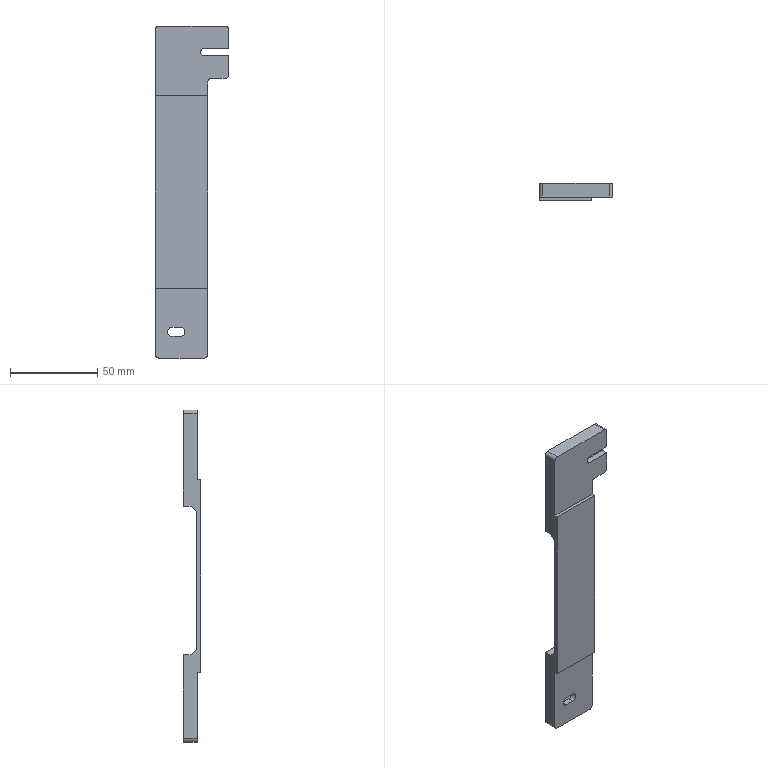Part | STEP file | 1 solid | 41 faces | box 42 x 10 x 190 mm | volume 34788 mm3 | plane 29 | cylinder 12 | commonest cylinder face diameters 4 x6 8 x3 5 x2 4.2 x1